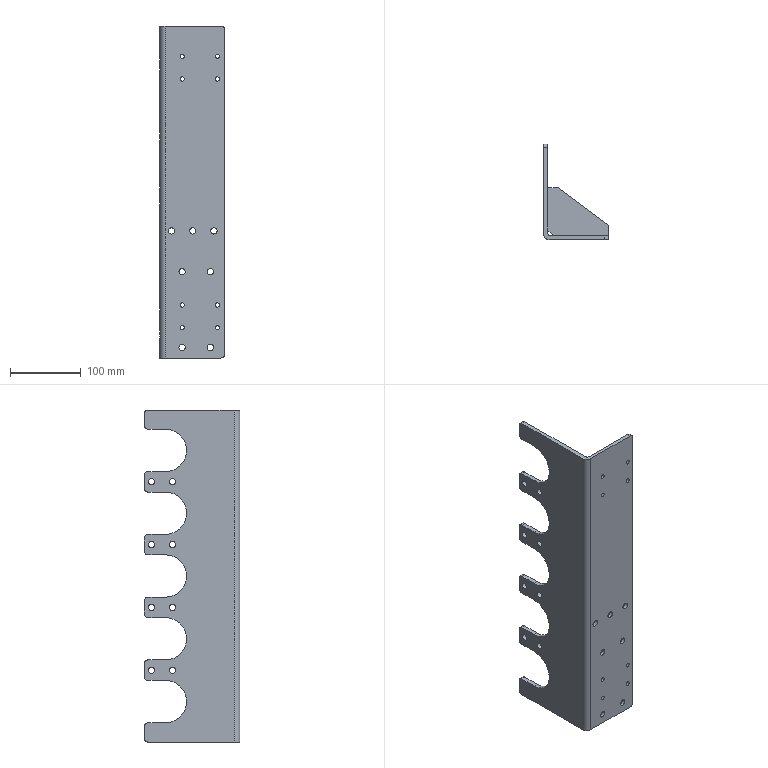Part | SolidWorks | features BaseBody 1 | 1 solid | 100 faces | box 92 x 135 x 470 mm | volume 514041 mm3 | cylinder 67 | plane 33 | commonest cylinder face diameters 9 x30 6 x16 10 x14 60 x5 8 x1 16 x1